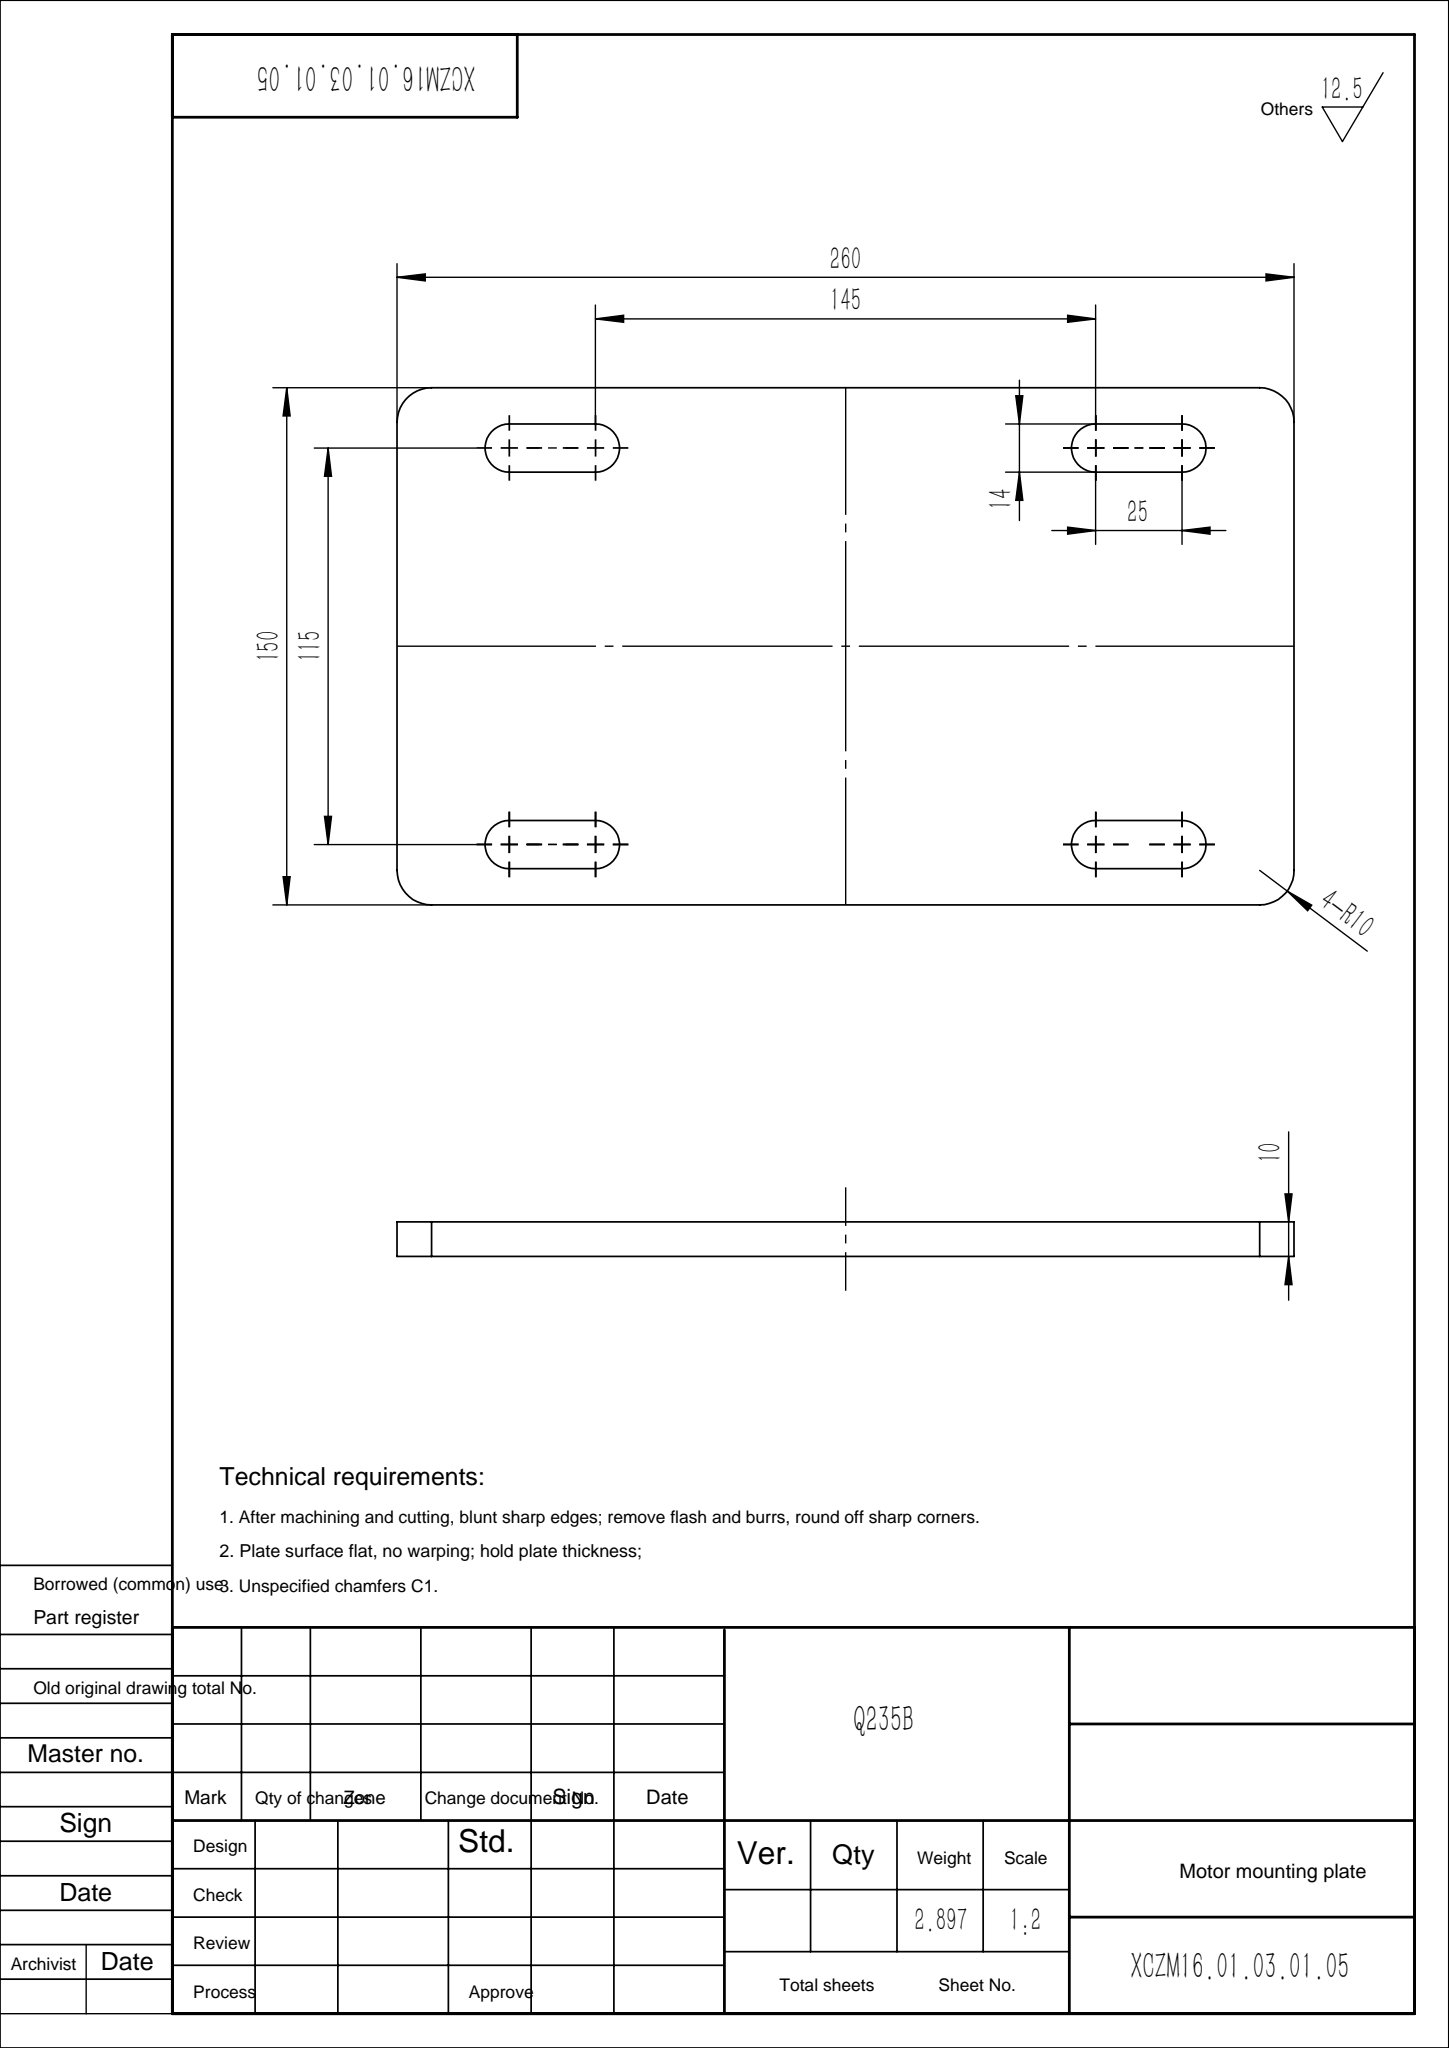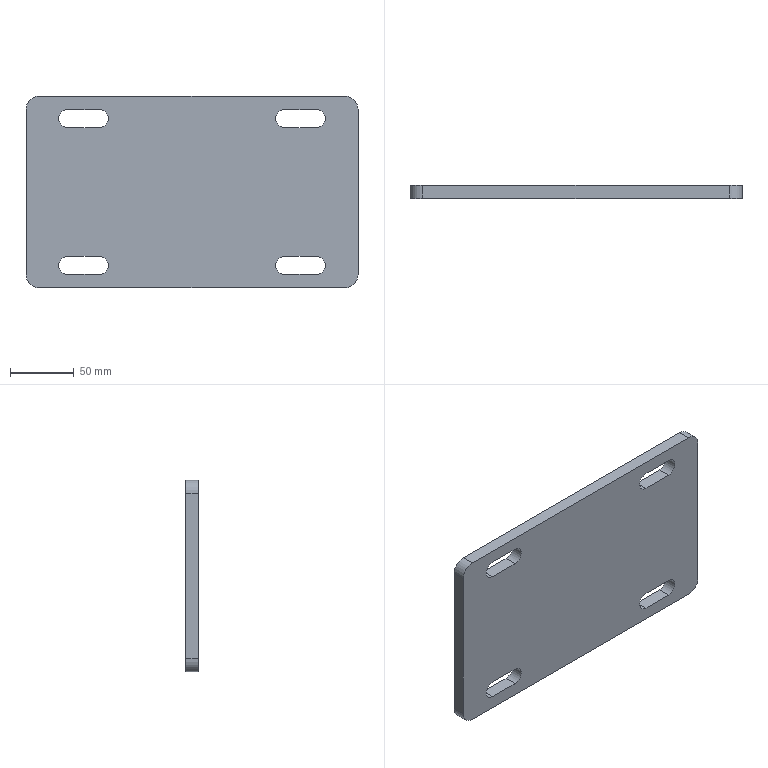Part | SolidWorks | features Extrusion 1 | 1 solid | 26 faces | box 260 x 10 x 150 mm | volume 368984 mm3 | plane 14 | cylinder 12 | commonest cylinder face diameters 14 x8 20 x4
STEP:
#1=CARTESIAN_POINT('',(-72.5,10.,64.5));
#2=VERTEX_POINT('',#1);
#3=CARTESIAN_POINT('',(-72.5,10.,50.5));
#4=VERTEX_POINT('',#3);
#5=CARTESIAN_POINT('',(-72.5,10.,57.5));
#6=DIRECTION('',(0.,1.,0.));
#7=DIRECTION('',(0.,0.,-1.));
#8=AXIS2_PLACEMENT_3D('',#5,#6,#7);
#9=CIRCLE('',#8,7.);
#10=EDGE_CURVE('',#2,#4,#9,.T.);
#11=ORIENTED_EDGE('',*,*,#10,.F.);
#12=CARTESIAN_POINT('',(-97.5,10.,64.5));
#13=VERTEX_POINT('',#12);
#14=CARTESIAN_POINT('',(-72.5,10.,64.5));
#15=DIRECTION('',(1.,0.,0.));
#16=VECTOR('',#15,1000.);
#17=LINE('',#14,#16);
#18=EDGE_CURVE('',#13,#2,#17,.T.);
#19=ORIENTED_EDGE('',*,*,#18,.F.);
#20=CARTESIAN_POINT('',(-97.5,10.,50.5));
#21=VERTEX_POINT('',#20);
#22=CARTESIAN_POINT('',(-97.5,10.,57.5));
#23=DIRECTION('',(0.,1.,0.));
#24=DIRECTION('',(0.,0.,-1.));
#25=AXIS2_PLACEMENT_3D('',#22,#23,#24);
#26=CIRCLE('',#25,7.);
#27=EDGE_CURVE('',#21,#13,#26,.T.);
#28=ORIENTED_EDGE('',*,*,#27,.F.);
#29=CARTESIAN_POINT('',(-72.5,10.,50.5));
#30=DIRECTION('',(-1.,0.,0.));
#31=VECTOR('',#30,1000.);
#32=LINE('',#29,#31);
#33=EDGE_CURVE('',#4,#21,#32,.T.);
#34=ORIENTED_EDGE('',*,*,#33,.F.);
#35=EDGE_LOOP('',(#11,#19,#28,#34));
#36=FACE_BOUND('',#35,.T.);
#37=CARTESIAN_POINT('',(-72.5,10.,-50.5));
#38=VERTEX_POINT('',#37);
#39=CARTESIAN_POINT('',(-72.5,10.,-64.5));
#40=VERTEX_POINT('',#39);
#41=CARTESIAN_POINT('',(-72.5,10.,-57.5));
#42=DIRECTION('',(0.,1.,0.));
#43=DIRECTION('',(0.,0.,1.));
#44=AXIS2_PLACEMENT_3D('',#41,#42,#43);
#45=CIRCLE('',#44,7.);
#46=EDGE_CURVE('',#38,#40,#45,.T.);
#47=ORIENTED_EDGE('',*,*,#46,.F.);
#48=CARTESIAN_POINT('',(-97.5,10.,-50.5));
#49=VERTEX_POINT('',#48);
#50=CARTESIAN_POINT('',(-72.5,10.,-50.5));
#51=DIRECTION('',(1.,0.,0.));
#52=VECTOR('',#51,1000.);
#53=LINE('',#50,#52);
#54=EDGE_CURVE('',#49,#38,#53,.T.);
#55=ORIENTED_EDGE('',*,*,#54,.F.);
#56=CARTESIAN_POINT('',(-97.5,10.,-64.5));
#57=VERTEX_POINT('',#56);
#58=CARTESIAN_POINT('',(-97.5,10.,-57.5));
#59=DIRECTION('',(0.,1.,0.));
#60=DIRECTION('',(0.,0.,1.));
#61=AXIS2_PLACEMENT_3D('',#58,#59,#60);
#62=CIRCLE('',#61,7.);
#63=EDGE_CURVE('',#57,#49,#62,.T.);
#64=ORIENTED_EDGE('',*,*,#63,.F.);
#65=CARTESIAN_POINT('',(-72.5,10.,-64.5));
#66=DIRECTION('',(-1.,0.,0.));
#67=VECTOR('',#66,1000.);
#68=LINE('',#65,#67);
#69=EDGE_CURVE('',#40,#57,#68,.T.);
#70=ORIENTED_EDGE('',*,*,#69,.F.);
#71=EDGE_LOOP('',(#47,#55,#64,#70));
#72=FACE_BOUND('',#71,.T.);
#73=CARTESIAN_POINT('',(-130.,10.,65.));
#74=VERTEX_POINT('',#73);
#75=CARTESIAN_POINT('',(-120.,10.,75.));
#76=VERTEX_POINT('',#75);
#77=CARTESIAN_POINT('',(-120.,10.,65.));
#78=DIRECTION('',(0.,1.,0.));
#79=DIRECTION('',(0.,0.,-1.));
#80=AXIS2_PLACEMENT_3D('',#77,#78,#79);
#81=CIRCLE('',#80,10.);
#82=EDGE_CURVE('',#74,#76,#81,.T.);
#83=ORIENTED_EDGE('',*,*,#82,.T.);
#84=CARTESIAN_POINT('',(120.,10.,75.));
#85=VERTEX_POINT('',#84);
#86=CARTESIAN_POINT('',(120.,10.,75.));
#87=DIRECTION('',(1.,0.,0.));
#88=VECTOR('',#87,1000.);
#89=LINE('',#86,#88);
#90=EDGE_CURVE('',#76,#85,#89,.T.);
#91=ORIENTED_EDGE('',*,*,#90,.T.);
#92=CARTESIAN_POINT('',(130.,10.,65.));
#93=VERTEX_POINT('',#92);
#94=CARTESIAN_POINT('',(120.,10.,65.));
#95=DIRECTION('',(0.,1.,0.));
#96=DIRECTION('',(0.,0.,1.));
#97=AXIS2_PLACEMENT_3D('',#94,#95,#96);
#98=CIRCLE('',#97,10.);
#99=EDGE_CURVE('',#85,#93,#98,.T.);
#100=ORIENTED_EDGE('',*,*,#99,.T.);
#101=CARTESIAN_POINT('',(130.,10.,-65.));
#102=VERTEX_POINT('',#101);
#103=CARTESIAN_POINT('',(130.,10.,65.));
#104=DIRECTION('',(0.,0.,-1.));
#105=VECTOR('',#104,1000.);
#106=LINE('',#103,#105);
#107=EDGE_CURVE('',#93,#102,#106,.T.);
#108=ORIENTED_EDGE('',*,*,#107,.T.);
#109=CARTESIAN_POINT('',(120.,10.,-75.));
#110=VERTEX_POINT('',#109);
#111=CARTESIAN_POINT('',(120.,10.,-65.));
#112=DIRECTION('',(0.,1.,0.));
#113=DIRECTION('',(0.,0.,1.));
#114=AXIS2_PLACEMENT_3D('',#111,#112,#113);
#115=CIRCLE('',#114,10.);
#116=EDGE_CURVE('',#102,#110,#115,.T.);
#117=ORIENTED_EDGE('',*,*,#116,.T.);
#118=CARTESIAN_POINT('',(-120.,10.,-75.));
#119=VERTEX_POINT('',#118);
#120=CARTESIAN_POINT('',(120.,10.,-75.));
#121=DIRECTION('',(-1.,0.,0.));
#122=VECTOR('',#121,1000.);
#123=LINE('',#120,#122);
#124=EDGE_CURVE('',#110,#119,#123,.T.);
#125=ORIENTED_EDGE('',*,*,#124,.T.);
#126=CARTESIAN_POINT('',(-130.,10.,-65.));
#127=VERTEX_POINT('',#126);
#128=CARTESIAN_POINT('',(-120.,10.,-65.));
#129=DIRECTION('',(0.,1.,0.));
#130=DIRECTION('',(0.,0.,1.));
#131=AXIS2_PLACEMENT_3D('',#128,#129,#130);
#132=CIRCLE('',#131,10.);
#133=EDGE_CURVE('',#119,#127,#132,.T.);
#134=ORIENTED_EDGE('',*,*,#133,.T.);
#135=CARTESIAN_POINT('',(-130.,10.,65.));
#136=DIRECTION('',(0.,0.,1.));
#137=VECTOR('',#136,1000.);
#138=LINE('',#135,#137);
#139=EDGE_CURVE('',#127,#74,#138,.T.);
#140=ORIENTED_EDGE('',*,*,#139,.T.);
#141=EDGE_LOOP('',(#83,#91,#100,#108,#117,#125,#134,#140));
#142=FACE_OUTER_BOUND('',#141,.T.);
#143=CARTESIAN_POINT('',(72.5,10.,-64.5));
#144=VERTEX_POINT('',#143);
#145=CARTESIAN_POINT('',(72.5,10.,-50.5));
#146=VERTEX_POINT('',#145);
#147=CARTESIAN_POINT('',(72.5,10.,-57.5));
#148=DIRECTION('',(0.,1.,0.));
#149=DIRECTION('',(0.,0.,-1.));
#150=AXIS2_PLACEMENT_3D('',#147,#148,#149);
#151=CIRCLE('',#150,7.);
#152=EDGE_CURVE('',#144,#146,#151,.T.);
#153=ORIENTED_EDGE('',*,*,#152,.F.);
#154=CARTESIAN_POINT('',(97.5,10.,-64.5));
#155=VERTEX_POINT('',#154);
#156=CARTESIAN_POINT('',(72.5,10.,-64.5));
#157=DIRECTION('',(-1.,0.,0.));
#158=VECTOR('',#157,1000.);
#159=LINE('',#156,#158);
#160=EDGE_CURVE('',#155,#144,#159,.T.);
#161=ORIENTED_EDGE('',*,*,#160,.F.);
#162=CARTESIAN_POINT('',(97.5,10.,-50.5));
#163=VERTEX_POINT('',#162);
#164=CARTESIAN_POINT('',(97.5,10.,-57.5));
#165=DIRECTION('',(0.,1.,0.));
#166=DIRECTION('',(0.,0.,-1.));
#167=AXIS2_PLACEMENT_3D('',#164,#165,#166);
#168=CIRCLE('',#167,7.);
#169=EDGE_CURVE('',#163,#155,#168,.T.);
#170=ORIENTED_EDGE('',*,*,#169,.F.);
#171=CARTESIAN_POINT('',(72.5,10.,-50.5));
#172=DIRECTION('',(1.,0.,0.));
#173=VECTOR('',#172,1000.);
#174=LINE('',#171,#173);
#175=EDGE_CURVE('',#146,#163,#174,.T.);
#176=ORIENTED_EDGE('',*,*,#175,.F.);
#177=EDGE_LOOP('',(#153,#161,#170,#176));
#178=FACE_BOUND('',#177,.T.);
#179=CARTESIAN_POINT('',(72.5,10.,50.5));
#180=VERTEX_POINT('',#179);
#181=CARTESIAN_POINT('',(72.5,10.,64.5));
#182=VERTEX_POINT('',#181);
#183=CARTESIAN_POINT('',(72.5,10.,57.5));
#184=DIRECTION('',(0.,1.,0.));
#185=DIRECTION('',(0.,0.,1.));
#186=AXIS2_PLACEMENT_3D('',#183,#184,#185);
#187=CIRCLE('',#186,7.);
#188=EDGE_CURVE('',#180,#182,#187,.T.);
#189=ORIENTED_EDGE('',*,*,#188,.F.);
#190=CARTESIAN_POINT('',(97.5,10.,50.5));
#191=VERTEX_POINT('',#190);
#192=CARTESIAN_POINT('',(72.5,10.,50.5));
#193=DIRECTION('',(-1.,0.,0.));
#194=VECTOR('',#193,1000.);
#195=LINE('',#192,#194);
#196=EDGE_CURVE('',#191,#180,#195,.T.);
#197=ORIENTED_EDGE('',*,*,#196,.F.);
#198=CARTESIAN_POINT('',(97.5,10.,64.5));
#199=VERTEX_POINT('',#198);
#200=CARTESIAN_POINT('',(97.5,10.,57.5));
#201=DIRECTION('',(0.,1.,0.));
#202=DIRECTION('',(0.,0.,1.));
#203=AXIS2_PLACEMENT_3D('',#200,#201,#202);
#204=CIRCLE('',#203,7.);
#205=EDGE_CURVE('',#199,#191,#204,.T.);
#206=ORIENTED_EDGE('',*,*,#205,.F.);
#207=CARTESIAN_POINT('',(72.5,10.,64.5));
#208=DIRECTION('',(1.,0.,0.));
#209=VECTOR('',#208,1000.);
#210=LINE('',#207,#209);
#211=EDGE_CURVE('',#182,#199,#210,.T.);
#212=ORIENTED_EDGE('',*,*,#211,.F.);
#213=EDGE_LOOP('',(#189,#197,#206,#212));
#214=FACE_BOUND('',#213,.T.);
#215=CARTESIAN_POINT('',(-120.,10.,65.));
#216=DIRECTION('',(0.,-1.,0.));
#217=DIRECTION('',(0.,0.,-1.));
#218=AXIS2_PLACEMENT_3D('',#215,#216,#217);
#219=PLANE('',#218);
#220=ADVANCED_FACE('',(#36,#72,#142,#178,#214),#219,.F.);
#221=CARTESIAN_POINT('',(-130.,0.,65.));
#222=VERTEX_POINT('',#221);
#223=CARTESIAN_POINT('',(-120.,0.,75.));
#224=VERTEX_POINT('',#223);
#225=CARTESIAN_POINT('',(-120.,0.,65.));
#226=DIRECTION('',(0.,1.,0.));
#227=DIRECTION('',(0.,0.,-1.));
#228=AXIS2_PLACEMENT_3D('',#225,#226,#227);
#229=CIRCLE('',#228,10.);
#230=EDGE_CURVE('',#222,#224,#229,.T.);
#231=ORIENTED_EDGE('',*,*,#230,.F.);
#232=CARTESIAN_POINT('',(-130.,0.,-65.));
#233=VERTEX_POINT('',#232);
#234=CARTESIAN_POINT('',(-130.,0.,65.));
#235=DIRECTION('',(0.,0.,1.));
#236=VECTOR('',#235,1000.);
#237=LINE('',#234,#236);
#238=EDGE_CURVE('',#233,#222,#237,.T.);
#239=ORIENTED_EDGE('',*,*,#238,.F.);
#240=CARTESIAN_POINT('',(-120.,0.,-75.));
#241=VERTEX_POINT('',#240);
#242=CARTESIAN_POINT('',(-120.,0.,-65.));
#243=DIRECTION('',(0.,1.,0.));
#244=DIRECTION('',(0.,0.,1.));
#245=AXIS2_PLACEMENT_3D('',#242,#243,#244);
#246=CIRCLE('',#245,10.);
#247=EDGE_CURVE('',#241,#233,#246,.T.);
#248=ORIENTED_EDGE('',*,*,#247,.F.);
#249=CARTESIAN_POINT('',(120.,0.,-75.));
#250=VERTEX_POINT('',#249);
#251=CARTESIAN_POINT('',(120.,0.,-75.));
#252=DIRECTION('',(-1.,0.,0.));
#253=VECTOR('',#252,1000.);
#254=LINE('',#251,#253);
#255=EDGE_CURVE('',#250,#241,#254,.T.);
#256=ORIENTED_EDGE('',*,*,#255,.F.);
#257=CARTESIAN_POINT('',(130.,0.,-65.));
#258=VERTEX_POINT('',#257);
#259=CARTESIAN_POINT('',(120.,0.,-65.));
#260=DIRECTION('',(0.,1.,0.));
#261=DIRECTION('',(0.,0.,1.));
#262=AXIS2_PLACEMENT_3D('',#259,#260,#261);
#263=CIRCLE('',#262,10.);
#264=EDGE_CURVE('',#258,#250,#263,.T.);
#265=ORIENTED_EDGE('',*,*,#264,.F.);
#266=CARTESIAN_POINT('',(130.,0.,65.));
#267=VERTEX_POINT('',#266);
#268=CARTESIAN_POINT('',(130.,0.,65.));
#269=DIRECTION('',(0.,0.,-1.));
#270=VECTOR('',#269,1000.);
#271=LINE('',#268,#270);
#272=EDGE_CURVE('',#267,#258,#271,.T.);
#273=ORIENTED_EDGE('',*,*,#272,.F.);
#274=CARTESIAN_POINT('',(120.,0.,75.));
#275=VERTEX_POINT('',#274);
#276=CARTESIAN_POINT('',(120.,0.,65.));
#277=DIRECTION('',(0.,1.,0.));
#278=DIRECTION('',(0.,0.,1.));
#279=AXIS2_PLACEMENT_3D('',#276,#277,#278);
#280=CIRCLE('',#279,10.);
#281=EDGE_CURVE('',#275,#267,#280,.T.);
#282=ORIENTED_EDGE('',*,*,#281,.F.);
#283=CARTESIAN_POINT('',(120.,0.,75.));
#284=DIRECTION('',(1.,0.,0.));
#285=VECTOR('',#284,1000.);
#286=LINE('',#283,#285);
#287=EDGE_CURVE('',#224,#275,#286,.T.);
#288=ORIENTED_EDGE('',*,*,#287,.F.);
#289=EDGE_LOOP('',(#231,#239,#248,#256,#265,#273,#282,#288));
#290=FACE_OUTER_BOUND('',#289,.T.);
#291=CARTESIAN_POINT('',(-97.5,0.,-50.5));
#292=VERTEX_POINT('',#291);
#293=CARTESIAN_POINT('',(-72.5,0.,-50.5));
#294=VERTEX_POINT('',#293);
#295=CARTESIAN_POINT('',(-72.5,0.,-50.5));
#296=DIRECTION('',(1.,0.,0.));
#297=VECTOR('',#296,1000.);
#298=LINE('',#295,#297);
#299=EDGE_CURVE('',#292,#294,#298,.T.);
#300=ORIENTED_EDGE('',*,*,#299,.T.);
#301=CARTESIAN_POINT('',(-72.5,0.,-64.5));
#302=VERTEX_POINT('',#301);
#303=CARTESIAN_POINT('',(-72.5,0.,-57.5));
#304=DIRECTION('',(0.,1.,0.));
#305=DIRECTION('',(0.,0.,1.));
#306=AXIS2_PLACEMENT_3D('',#303,#304,#305);
#307=CIRCLE('',#306,7.);
#308=EDGE_CURVE('',#294,#302,#307,.T.);
#309=ORIENTED_EDGE('',*,*,#308,.T.);
#310=CARTESIAN_POINT('',(-97.5,0.,-64.5));
#311=VERTEX_POINT('',#310);
#312=CARTESIAN_POINT('',(-72.5,0.,-64.5));
#313=DIRECTION('',(-1.,0.,0.));
#314=VECTOR('',#313,1000.);
#315=LINE('',#312,#314);
#316=EDGE_CURVE('',#302,#311,#315,.T.);
#317=ORIENTED_EDGE('',*,*,#316,.T.);
#318=CARTESIAN_POINT('',(-97.5,0.,-57.5));
#319=DIRECTION('',(0.,1.,0.));
#320=DIRECTION('',(0.,0.,1.));
#321=AXIS2_PLACEMENT_3D('',#318,#319,#320);
#322=CIRCLE('',#321,7.);
#323=EDGE_CURVE('',#311,#292,#322,.T.);
#324=ORIENTED_EDGE('',*,*,#323,.T.);
#325=EDGE_LOOP('',(#300,#309,#317,#324));
#326=FACE_BOUND('',#325,.T.);
#327=CARTESIAN_POINT('',(97.5,0.,-64.5));
#328=VERTEX_POINT('',#327);
#329=CARTESIAN_POINT('',(72.5,0.,-64.5));
#330=VERTEX_POINT('',#329);
#331=CARTESIAN_POINT('',(72.5,0.,-64.5));
#332=DIRECTION('',(-1.,0.,0.));
#333=VECTOR('',#332,1000.);
#334=LINE('',#331,#333);
#335=EDGE_CURVE('',#328,#330,#334,.T.);
#336=ORIENTED_EDGE('',*,*,#335,.T.);
#337=CARTESIAN_POINT('',(72.5,0.,-50.5));
#338=VERTEX_POINT('',#337);
#339=CARTESIAN_POINT('',(72.5,0.,-57.5));
#340=DIRECTION('',(0.,1.,0.));
#341=DIRECTION('',(0.,0.,-1.));
#342=AXIS2_PLACEMENT_3D('',#339,#340,#341);
#343=CIRCLE('',#342,7.);
#344=EDGE_CURVE('',#330,#338,#343,.T.);
#345=ORIENTED_EDGE('',*,*,#344,.T.);
#346=CARTESIAN_POINT('',(97.5,0.,-50.5));
#347=VERTEX_POINT('',#346);
#348=CARTESIAN_POINT('',(72.5,0.,-50.5));
#349=DIRECTION('',(1.,0.,0.));
#350=VECTOR('',#349,1000.);
#351=LINE('',#348,#350);
#352=EDGE_CURVE('',#338,#347,#351,.T.);
#353=ORIENTED_EDGE('',*,*,#352,.T.);
#354=CARTESIAN_POINT('',(97.5,0.,-57.5));
#355=DIRECTION('',(0.,1.,0.));
#356=DIRECTION('',(0.,0.,-1.));
#357=AXIS2_PLACEMENT_3D('',#354,#355,#356);
#358=CIRCLE('',#357,7.);
#359=EDGE_CURVE('',#347,#328,#358,.T.);
#360=ORIENTED_EDGE('',*,*,#359,.T.);
#361=EDGE_LOOP('',(#336,#345,#353,#360));
#362=FACE_BOUND('',#361,.T.);
#363=CARTESIAN_POINT('',(-97.5,0.,64.5));
#364=VERTEX_POINT('',#363);
#365=CARTESIAN_POINT('',(-72.5,0.,64.5));
#366=VERTEX_POINT('',#365);
#367=CARTESIAN_POINT('',(-72.5,0.,64.5));
#368=DIRECTION('',(1.,0.,0.));
#369=VECTOR('',#368,1000.);
#370=LINE('',#367,#369);
#371=EDGE_CURVE('',#364,#366,#370,.T.);
#372=ORIENTED_EDGE('',*,*,#371,.T.);
#373=CARTESIAN_POINT('',(-72.5,0.,50.5));
#374=VERTEX_POINT('',#373);
#375=CARTESIAN_POINT('',(-72.5,0.,57.5));
#376=DIRECTION('',(0.,1.,0.));
#377=DIRECTION('',(0.,0.,-1.));
#378=AXIS2_PLACEMENT_3D('',#375,#376,#377);
#379=CIRCLE('',#378,7.);
#380=EDGE_CURVE('',#366,#374,#379,.T.);
#381=ORIENTED_EDGE('',*,*,#380,.T.);
#382=CARTESIAN_POINT('',(-97.5,0.,50.5));
#383=VERTEX_POINT('',#382);
#384=CARTESIAN_POINT('',(-72.5,0.,50.5));
#385=DIRECTION('',(-1.,0.,0.));
#386=VECTOR('',#385,1000.);
#387=LINE('',#384,#386);
#388=EDGE_CURVE('',#374,#383,#387,.T.);
#389=ORIENTED_EDGE('',*,*,#388,.T.);
#390=CARTESIAN_POINT('',(-97.5,0.,57.5));
#391=DIRECTION('',(0.,1.,0.));
#392=DIRECTION('',(0.,0.,-1.));
#393=AXIS2_PLACEMENT_3D('',#390,#391,#392);
#394=CIRCLE('',#393,7.);
#395=EDGE_CURVE('',#383,#364,#394,.T.);
#396=ORIENTED_EDGE('',*,*,#395,.T.);
#397=EDGE_LOOP('',(#372,#381,#389,#396));
#398=FACE_BOUND('',#397,.T.);
#399=CARTESIAN_POINT('',(97.5,0.,50.5));
#400=VERTEX_POINT('',#399);
#401=CARTESIAN_POINT('',(72.5,0.,50.5));
#402=VERTEX_POINT('',#401);
#403=CARTESIAN_POINT('',(72.5,0.,50.5));
#404=DIRECTION('',(-1.,0.,0.));
#405=VECTOR('',#404,1000.);
#406=LINE('',#403,#405);
#407=EDGE_CURVE('',#400,#402,#406,.T.);
#408=ORIENTED_EDGE('',*,*,#407,.T.);
#409=CARTESIAN_POINT('',(72.5,0.,64.5));
#410=VERTEX_POINT('',#409);
#411=CARTESIAN_POINT('',(72.5,0.,57.5));
#412=DIRECTION('',(0.,1.,0.));
#413=DIRECTION('',(0.,0.,1.));
#414=AXIS2_PLACEMENT_3D('',#411,#412,#413);
#415=CIRCLE('',#414,7.);
#416=EDGE_CURVE('',#402,#410,#415,.T.);
#417=ORIENTED_EDGE('',*,*,#416,.T.);
#418=CARTESIAN_POINT('',(97.5,0.,64.5));
#419=VERTEX_POINT('',#418);
#420=CARTESIAN_POINT('',(72.5,0.,64.5));
#421=DIRECTION('',(1.,0.,0.));
#422=VECTOR('',#421,1000.);
#423=LINE('',#420,#422);
#424=EDGE_CURVE('',#410,#419,#423,.T.);
#425=ORIENTED_EDGE('',*,*,#424,.T.);
#426=CARTESIAN_POINT('',(97.5,0.,57.5));
#427=DIRECTION('',(0.,1.,0.));
#428=DIRECTION('',(0.,0.,1.));
#429=AXIS2_PLACEMENT_3D('',#426,#427,#428);
#430=CIRCLE('',#429,7.);
#431=EDGE_CURVE('',#419,#400,#430,.T.);
#432=ORIENTED_EDGE('',*,*,#431,.T.);
#433=EDGE_LOOP('',(#408,#417,#425,#432));
#434=FACE_BOUND('',#433,.T.);
#435=CARTESIAN_POINT('',(-120.,0.,65.));
#436=DIRECTION('',(0.,-1.,0.));
#437=DIRECTION('',(0.,0.,-1.));
#438=AXIS2_PLACEMENT_3D('',#435,#436,#437);
#439=PLANE('',#438);
#440=ADVANCED_FACE('',(#290,#326,#362,#398,#434),#439,.T.);
#441=ORIENTED_EDGE('',*,*,#230,.T.);
#442=CARTESIAN_POINT('',(-120.,10.,75.));
#443=DIRECTION('',(0.,-1.,0.));
#444=VECTOR('',#443,1000.);
#445=LINE('',#442,#444);
#446=EDGE_CURVE('',#76,#224,#445,.T.);
#447=ORIENTED_EDGE('',*,*,#446,.F.);
#448=ORIENTED_EDGE('',*,*,#82,.F.);
#449=CARTESIAN_POINT('',(-130.,10.,65.));
#450=DIRECTION('',(0.,-1.,0.));
#451=VECTOR('',#450,1000.);
#452=LINE('',#449,#451);
#453=EDGE_CURVE('',#74,#222,#452,.T.);
#454=ORIENTED_EDGE('',*,*,#453,.T.);
#455=EDGE_LOOP('',(#441,#447,#448,#454));
#456=FACE_OUTER_BOUND('',#455,.T.);
#457=CARTESIAN_POINT('',(-120.,10.,65.));
#458=DIRECTION('',(0.,-1.,0.));
#459=DIRECTION('',(0.,0.,-1.));
#460=AXIS2_PLACEMENT_3D('',#457,#458,#459);
#461=CYLINDRICAL_SURFACE('',#460,10.);
#462=ADVANCED_FACE('',(#456),#461,.T.);
#463=ORIENTED_EDGE('',*,*,#287,.T.);
#464=CARTESIAN_POINT('',(120.,10.,75.));
#465=DIRECTION('',(0.,-1.,0.));
#466=VECTOR('',#465,1000.);
#467=LINE('',#464,#466);
#468=EDGE_CURVE('',#85,#275,#467,.T.);
#469=ORIENTED_EDGE('',*,*,#468,.F.);
#470=ORIENTED_EDGE('',*,*,#90,.F.);
#471=ORIENTED_EDGE('',*,*,#446,.T.);
#472=EDGE_LOOP('',(#463,#469,#470,#471));
#473=FACE_OUTER_BOUND('',#472,.T.);
#474=CARTESIAN_POINT('',(120.,10.,75.));
#475=DIRECTION('',(0.,0.,-1.));
#476=DIRECTION('',(-1.,0.,0.));
#477=AXIS2_PLACEMENT_3D('',#474,#475,#476);
#478=PLANE('',#477);
#479=ADVANCED_FACE('',(#473),#478,.F.);
#480=ORIENTED_EDGE('',*,*,#281,.T.);
#481=CARTESIAN_POINT('',(130.,10.,65.));
#482=DIRECTION('',(0.,-1.,0.));
#483=VECTOR('',#482,1000.);
#484=LINE('',#481,#483);
#485=EDGE_CURVE('',#93,#267,#484,.T.);
#486=ORIENTED_EDGE('',*,*,#485,.F.);
#487=ORIENTED_EDGE('',*,*,#99,.F.);
#488=ORIENTED_EDGE('',*,*,#468,.T.);
#489=EDGE_LOOP('',(#480,#486,#487,#488));
#490=FACE_OUTER_BOUND('',#489,.T.);
#491=CARTESIAN_POINT('',(120.,10.,65.));
#492=DIRECTION('',(0.,-1.,0.));
#493=DIRECTION('',(0.,0.,-1.));
#494=AXIS2_PLACEMENT_3D('',#491,#492,#493);
#495=CYLINDRICAL_SURFACE('',#494,10.);
#496=ADVANCED_FACE('',(#490),#495,.T.);
#497=ORIENTED_EDGE('',*,*,#272,.T.);
#498=CARTESIAN_POINT('',(130.,10.,-65.));
#499=DIRECTION('',(0.,-1.,0.));
#500=VECTOR('',#499,1000.);
#501=LINE('',#498,#500);
#502=EDGE_CURVE('',#102,#258,#501,.T.);
#503=ORIENTED_EDGE('',*,*,#502,.F.);
#504=ORIENTED_EDGE('',*,*,#107,.F.);
#505=ORIENTED_EDGE('',*,*,#485,.T.);
#506=EDGE_LOOP('',(#497,#503,#504,#505));
#507=FACE_OUTER_BOUND('',#506,.T.);
#508=CARTESIAN_POINT('',(130.,10.,65.));
#509=DIRECTION('',(-1.,0.,0.));
#510=DIRECTION('',(0.,0.,1.));
#511=AXIS2_PLACEMENT_3D('',#508,#509,#510);
#512=PLANE('',#511);
#513=ADVANCED_FACE('',(#507),#512,.F.);
#514=ORIENTED_EDGE('',*,*,#264,.T.);
#515=CARTESIAN_POINT('',(120.,10.,-75.));
#516=DIRECTION('',(0.,-1.,0.));
#517=VECTOR('',#516,1000.);
#518=LINE('',#515,#517);
#519=EDGE_CURVE('',#110,#250,#518,.T.);
#520=ORIENTED_EDGE('',*,*,#519,.F.);
#521=ORIENTED_EDGE('',*,*,#116,.F.);
#522=ORIENTED_EDGE('',*,*,#502,.T.);
#523=EDGE_LOOP('',(#514,#520,#521,#522));
#524=FACE_OUTER_BOUND('',#523,.T.);
#525=CARTESIAN_POINT('',(120.,10.,-65.));
#526=DIRECTION('',(0.,-1.,0.));
#527=DIRECTION('',(0.,0.,-1.));
#528=AXIS2_PLACEMENT_3D('',#525,#526,#527);
#529=CYLINDRICAL_SURFACE('',#528,10.);
#530=ADVANCED_FACE('',(#524),#529,.T.);
#531=ORIENTED_EDGE('',*,*,#255,.T.);
#532=CARTESIAN_POINT('',(-120.,10.,-75.));
#533=DIRECTION('',(0.,-1.,0.));
#534=VECTOR('',#533,1000.);
#535=LINE('',#532,#534);
#536=EDGE_CURVE('',#119,#241,#535,.T.);
#537=ORIENTED_EDGE('',*,*,#536,.F.);
#538=ORIENTED_EDGE('',*,*,#124,.F.);
#539=ORIENTED_EDGE('',*,*,#519,.T.);
#540=EDGE_LOOP('',(#531,#537,#538,#539));
#541=FACE_OUTER_BOUND('',#540,.T.);
#542=CARTESIAN_POINT('',(120.,10.,-75.));
#543=DIRECTION('',(0.,0.,1.));
#544=DIRECTION('',(1.,0.,0.));
#545=AXIS2_PLACEMENT_3D('',#542,#543,#544);
#546=PLANE('',#545);
#547=ADVANCED_FACE('',(#541),#546,.F.);
#548=ORIENTED_EDGE('',*,*,#247,.T.);
#549=CARTESIAN_POINT('',(-130.,10.,-65.));
#550=DIRECTION('',(0.,-1.,0.));
#551=VECTOR('',#550,1000.);
#552=LINE('',#549,#551);
#553=EDGE_CURVE('',#127,#233,#552,.T.);
#554=ORIENTED_EDGE('',*,*,#553,.F.);
#555=ORIENTED_EDGE('',*,*,#133,.F.);
#556=ORIENTED_EDGE('',*,*,#536,.T.);
#557=EDGE_LOOP('',(#548,#554,#555,#556));
#558=FACE_OUTER_BOUND('',#557,.T.);
#559=CARTESIAN_POINT('',(-120.,10.,-65.));
#560=DIRECTION('',(0.,-1.,0.));
#561=DIRECTION('',(0.,0.,-1.));
#562=AXIS2_PLACEMENT_3D('',#559,#560,#561);
#563=CYLINDRICAL_SURFACE('',#562,10.);
#564=ADVANCED_FACE('',(#558),#563,.T.);
#565=ORIENTED_EDGE('',*,*,#238,.T.);
#566=ORIENTED_EDGE('',*,*,#453,.F.);
#567=ORIENTED_EDGE('',*,*,#139,.F.);
#568=ORIENTED_EDGE('',*,*,#553,.T.);
#569=EDGE_LOOP('',(#565,#566,#567,#568));
#570=FACE_OUTER_BOUND('',#569,.T.);
#571=CARTESIAN_POINT('',(-130.,10.,65.));
#572=DIRECTION('',(1.,0.,0.));
#573=DIRECTION('',(0.,0.,-1.));
#574=AXIS2_PLACEMENT_3D('',#571,#572,#573);
#575=PLANE('',#574);
#576=ADVANCED_FACE('',(#570),#575,.F.);
#577=ORIENTED_EDGE('',*,*,#308,.F.);
#578=CARTESIAN_POINT('',(-72.5,10.,-50.5));
#579=DIRECTION('',(0.,-1.,0.));
#580=VECTOR('',#579,1000.);
#581=LINE('',#578,#580);
#582=EDGE_CURVE('',#38,#294,#581,.T.);
#583=ORIENTED_EDGE('',*,*,#582,.F.);
#584=ORIENTED_EDGE('',*,*,#46,.T.);
#585=CARTESIAN_POINT('',(-72.5,10.,-64.5));
#586=DIRECTION('',(0.,-1.,0.));
#587=VECTOR('',#586,1000.);
#588=LINE('',#585,#587);
#589=EDGE_CURVE('',#40,#302,#588,.T.);
#590=ORIENTED_EDGE('',*,*,#589,.T.);
#591=EDGE_LOOP('',(#577,#583,#584,#590));
#592=FACE_OUTER_BOUND('',#591,.T.);
#593=CARTESIAN_POINT('',(-72.5,10.,-57.5));
#594=DIRECTION('',(0.,-1.,0.));
#595=DIRECTION('',(0.,0.,-1.));
#596=AXIS2_PLACEMENT_3D('',#593,#594,#595);
#597=CYLINDRICAL_SURFACE('',#596,7.);
#598=ADVANCED_FACE('',(#592),#597,.F.);
#599=ORIENTED_EDGE('',*,*,#316,.F.);
#600=ORIENTED_EDGE('',*,*,#589,.F.);
#601=ORIENTED_EDGE('',*,*,#69,.T.);
#602=CARTESIAN_POINT('',(-97.5,10.,-64.5));
#603=DIRECTION('',(0.,-1.,0.));
#604=VECTOR('',#603,1000.);
#605=LINE('',#602,#604);
#606=EDGE_CURVE('',#57,#311,#605,.T.);
#607=ORIENTED_EDGE('',*,*,#606,.T.);
#608=EDGE_LOOP('',(#599,#600,#601,#607));
#609=FACE_OUTER_BOUND('',#608,.T.);
#610=CARTESIAN_POINT('',(-72.5,10.,-64.5));
#611=DIRECTION('',(0.,0.,1.));
#612=DIRECTION('',(1.,0.,0.));
#613=AXIS2_PLACEMENT_3D('',#610,#611,#612);
#614=PLANE('',#613);
#615=ADVANCED_FACE('',(#609),#614,.T.);
#616=ORIENTED_EDGE('',*,*,#323,.F.);
#617=ORIENTED_EDGE('',*,*,#606,.F.);
#618=ORIENTED_EDGE('',*,*,#63,.T.);
#619=CARTESIAN_POINT('',(-97.5,10.,-50.5));
#620=DIRECTION('',(0.,-1.,0.));
#621=VECTOR('',#620,1000.);
#622=LINE('',#619,#621);
#623=EDGE_CURVE('',#49,#292,#622,.T.);
#624=ORIENTED_EDGE('',*,*,#623,.T.);
#625=EDGE_LOOP('',(#616,#617,#618,#624));
#626=FACE_OUTER_BOUND('',#625,.T.);
#627=CARTESIAN_POINT('',(-97.5,10.,-57.5));
#628=DIRECTION('',(0.,-1.,0.));
#629=DIRECTION('',(0.,0.,-1.));
#630=AXIS2_PLACEMENT_3D('',#627,#628,#629);
#631=CYLINDRICAL_SURFACE('',#630,7.);
#632=ADVANCED_FACE('',(#626),#631,.F.);
#633=ORIENTED_EDGE('',*,*,#299,.F.);
#634=ORIENTED_EDGE('',*,*,#623,.F.);
#635=ORIENTED_EDGE('',*,*,#54,.T.);
#636=ORIENTED_EDGE('',*,*,#582,.T.);
#637=EDGE_LOOP('',(#633,#634,#635,#636));
#638=FACE_OUTER_BOUND('',#637,.T.);
#639=CARTESIAN_POINT('',(-72.5,10.,-50.5));
#640=DIRECTION('',(0.,0.,-1.));
#641=DIRECTION('',(-1.,0.,0.));
#642=AXIS2_PLACEMENT_3D('',#639,#640,#641);
#643=PLANE('',#642);
#644=ADVANCED_FACE('',(#638),#643,.T.);
#645=ORIENTED_EDGE('',*,*,#344,.F.);
#646=CARTESIAN_POINT('',(72.5,10.,-64.5));
#647=DIRECTION('',(0.,-1.,0.));
#648=VECTOR('',#647,1000.);
#649=LINE('',#646,#648);
#650=EDGE_CURVE('',#144,#330,#649,.T.);
#651=ORIENTED_EDGE('',*,*,#650,.F.);
#652=ORIENTED_EDGE('',*,*,#152,.T.);
#653=CARTESIAN_POINT('',(72.5,10.,-50.5));
#654=DIRECTION('',(0.,-1.,0.));
#655=VECTOR('',#654,1000.);
#656=LINE('',#653,#655);
#657=EDGE_CURVE('',#146,#338,#656,.T.);
#658=ORIENTED_EDGE('',*,*,#657,.T.);
#659=EDGE_LOOP('',(#645,#651,#652,#658));
#660=FACE_OUTER_BOUND('',#659,.T.);
#661=CARTESIAN_POINT('',(72.5,10.,-57.5));
#662=DIRECTION('',(0.,-1.,0.));
#663=DIRECTION('',(0.,0.,-1.));
#664=AXIS2_PLACEMENT_3D('',#661,#662,#663);
#665=CYLINDRICAL_SURFACE('',#664,7.);
#666=ADVANCED_FACE('',(#660),#665,.F.);
#667=ORIENTED_EDGE('',*,*,#352,.F.);
#668=ORIENTED_EDGE('',*,*,#657,.F.);
#669=ORIENTED_EDGE('',*,*,#175,.T.);
#670=CARTESIAN_POINT('',(97.5,10.,-50.5));
#671=DIRECTION('',(0.,-1.,0.));
#672=VECTOR('',#671,1000.);
#673=LINE('',#670,#672);
#674=EDGE_CURVE('',#163,#347,#673,.T.);
#675=ORIENTED_EDGE('',*,*,#674,.T.);
#676=EDGE_LOOP('',(#667,#668,#669,#675));
#677=FACE_OUTER_BOUND('',#676,.T.);
#678=CARTESIAN_POINT('',(72.5,10.,-50.5));
#679=DIRECTION('',(0.,0.,-1.));
#680=DIRECTION('',(-1.,0.,0.));
#681=AXIS2_PLACEMENT_3D('',#678,#679,#680);
#682=PLANE('',#681);
#683=ADVANCED_FACE('',(#677),#682,.T.);
#684=ORIENTED_EDGE('',*,*,#359,.F.);
#685=ORIENTED_EDGE('',*,*,#674,.F.);
#686=ORIENTED_EDGE('',*,*,#169,.T.);
#687=CARTESIAN_POINT('',(97.5,10.,-64.5));
#688=DIRECTION('',(0.,-1.,0.));
#689=VECTOR('',#688,1000.);
#690=LINE('',#687,#689);
#691=EDGE_CURVE('',#155,#328,#690,.T.);
#692=ORIENTED_EDGE('',*,*,#691,.T.);
#693=EDGE_LOOP('',(#684,#685,#686,#692));
#694=FACE_OUTER_BOUND('',#693,.T.);
#695=CARTESIAN_POINT('',(97.5,10.,-57.5));
#696=DIRECTION('',(0.,-1.,0.));
#697=DIRECTION('',(0.,0.,-1.));
#698=AXIS2_PLACEMENT_3D('',#695,#696,#697);
#699=CYLINDRICAL_SURFACE('',#698,7.);
#700=ADVANCED_FACE('',(#694),#699,.F.);
#701=ORIENTED_EDGE('',*,*,#335,.F.);
#702=ORIENTED_EDGE('',*,*,#691,.F.);
#703=ORIENTED_EDGE('',*,*,#160,.T.);
#704=ORIENTED_EDGE('',*,*,#650,.T.);
#705=EDGE_LOOP('',(#701,#702,#703,#704));
#706=FACE_OUTER_BOUND('',#705,.T.);
#707=CARTESIAN_POINT('',(72.5,10.,-64.5));
#708=DIRECTION('',(0.,0.,1.));
#709=DIRECTION('',(1.,0.,0.));
#710=AXIS2_PLACEMENT_3D('',#707,#708,#709);
#711=PLANE('',#710);
#712=ADVANCED_FACE('',(#706),#711,.T.);
#713=ORIENTED_EDGE('',*,*,#380,.F.);
#714=CARTESIAN_POINT('',(-72.5,10.,64.5));
#715=DIRECTION('',(0.,-1.,0.));
#716=VECTOR('',#715,1000.);
#717=LINE('',#714,#716);
#718=EDGE_CURVE('',#2,#366,#717,.T.);
#719=ORIENTED_EDGE('',*,*,#718,.F.);
#720=ORIENTED_EDGE('',*,*,#10,.T.);
#721=CARTESIAN_POINT('',(-72.5,10.,50.5));
#722=DIRECTION('',(0.,-1.,0.));
#723=VECTOR('',#722,1000.);
#724=LINE('',#721,#723);
#725=EDGE_CURVE('',#4,#374,#724,.T.);
#726=ORIENTED_EDGE('',*,*,#725,.T.);
#727=EDGE_LOOP('',(#713,#719,#720,#726));
#728=FACE_OUTER_BOUND('',#727,.T.);
#729=CARTESIAN_POINT('',(-72.5,10.,57.5));
#730=DIRECTION('',(0.,-1.,0.));
#731=DIRECTION('',(0.,0.,-1.));
#732=AXIS2_PLACEMENT_3D('',#729,#730,#731);
#733=CYLINDRICAL_SURFACE('',#732,7.);
#734=ADVANCED_FACE('',(#728),#733,.F.);
#735=ORIENTED_EDGE('',*,*,#388,.F.);
#736=ORIENTED_EDGE('',*,*,#725,.F.);
#737=ORIENTED_EDGE('',*,*,#33,.T.);
#738=CARTESIAN_POINT('',(-97.5,10.,50.5));
#739=DIRECTION('',(0.,-1.,0.));
#740=VECTOR('',#739,1000.);
#741=LINE('',#738,#740);
#742=EDGE_CURVE('',#21,#383,#741,.T.);
#743=ORIENTED_EDGE('',*,*,#742,.T.);
#744=EDGE_LOOP('',(#735,#736,#737,#743));
#745=FACE_OUTER_BOUND('',#744,.T.);
#746=CARTESIAN_POINT('',(-72.5,10.,50.5));
#747=DIRECTION('',(0.,0.,1.));
#748=DIRECTION('',(1.,0.,0.));
#749=AXIS2_PLACEMENT_3D('',#746,#747,#748);
#750=PLANE('',#749);
#751=ADVANCED_FACE('',(#745),#750,.T.);
#752=ORIENTED_EDGE('',*,*,#395,.F.);
#753=ORIENTED_EDGE('',*,*,#742,.F.);
#754=ORIENTED_EDGE('',*,*,#27,.T.);
#755=CARTESIAN_POINT('',(-97.5,10.,64.5));
#756=DIRECTION('',(0.,-1.,0.));
#757=VECTOR('',#756,1000.);
#758=LINE('',#755,#757);
#759=EDGE_CURVE('',#13,#364,#758,.T.);
#760=ORIENTED_EDGE('',*,*,#759,.T.);
#761=EDGE_LOOP('',(#752,#753,#754,#760));
#762=FACE_OUTER_BOUND('',#761,.T.);
#763=CARTESIAN_POINT('',(-97.5,10.,57.5));
#764=DIRECTION('',(0.,-1.,0.));
#765=DIRECTION('',(0.,0.,-1.));
#766=AXIS2_PLACEMENT_3D('',#763,#764,#765);
#767=CYLINDRICAL_SURFACE('',#766,7.);
#768=ADVANCED_FACE('',(#762),#767,.F.);
#769=ORIENTED_EDGE('',*,*,#371,.F.);
#770=ORIENTED_EDGE('',*,*,#759,.F.);
#771=ORIENTED_EDGE('',*,*,#18,.T.);
#772=ORIENTED_EDGE('',*,*,#718,.T.);
#773=EDGE_LOOP('',(#769,#770,#771,#772));
#774=FACE_OUTER_BOUND('',#773,.T.);
#775=CARTESIAN_POINT('',(-72.5,10.,64.5));
#776=DIRECTION('',(0.,0.,-1.));
#777=DIRECTION('',(-1.,0.,0.));
#778=AXIS2_PLACEMENT_3D('',#775,#776,#777);
#779=PLANE('',#778);
#780=ADVANCED_FACE('',(#774),#779,.T.);
#781=ORIENTED_EDGE('',*,*,#416,.F.);
#782=CARTESIAN_POINT('',(72.5,10.,50.5));
#783=DIRECTION('',(0.,-1.,0.));
#784=VECTOR('',#783,1000.);
#785=LINE('',#782,#784);
#786=EDGE_CURVE('',#180,#402,#785,.T.);
#787=ORIENTED_EDGE('',*,*,#786,.F.);
#788=ORIENTED_EDGE('',*,*,#188,.T.);
#789=CARTESIAN_POINT('',(72.5,10.,64.5));
#790=DIRECTION('',(0.,-1.,0.));
#791=VECTOR('',#790,1000.);
#792=LINE('',#789,#791);
#793=EDGE_CURVE('',#182,#410,#792,.T.);
#794=ORIENTED_EDGE('',*,*,#793,.T.);
#795=EDGE_LOOP('',(#781,#787,#788,#794));
#796=FACE_OUTER_BOUND('',#795,.T.);
#797=CARTESIAN_POINT('',(72.5,10.,57.5));
#798=DIRECTION('',(0.,-1.,0.));
#799=DIRECTION('',(0.,0.,-1.));
#800=AXIS2_PLACEMENT_3D('',#797,#798,#799);
#801=CYLINDRICAL_SURFACE('',#800,7.);
#802=ADVANCED_FACE('',(#796),#801,.F.);
#803=ORIENTED_EDGE('',*,*,#424,.F.);
#804=ORIENTED_EDGE('',*,*,#793,.F.);
#805=ORIENTED_EDGE('',*,*,#211,.T.);
#806=CARTESIAN_POINT('',(97.5,10.,64.5));
#807=DIRECTION('',(0.,-1.,0.));
#808=VECTOR('',#807,1000.);
#809=LINE('',#806,#808);
#810=EDGE_CURVE('',#199,#419,#809,.T.);
#811=ORIENTED_EDGE('',*,*,#810,.T.);
#812=EDGE_LOOP('',(#803,#804,#805,#811));
#813=FACE_OUTER_BOUND('',#812,.T.);
#814=CARTESIAN_POINT('',(72.5,10.,64.5));
#815=DIRECTION('',(0.,0.,-1.));
#816=DIRECTION('',(-1.,0.,0.));
#817=AXIS2_PLACEMENT_3D('',#814,#815,#816);
#818=PLANE('',#817);
#819=ADVANCED_FACE('',(#813),#818,.T.);
#820=ORIENTED_EDGE('',*,*,#431,.F.);
#821=ORIENTED_EDGE('',*,*,#810,.F.);
#822=ORIENTED_EDGE('',*,*,#205,.T.);
#823=CARTESIAN_POINT('',(97.5,10.,50.5));
#824=DIRECTION('',(0.,-1.,0.));
#825=VECTOR('',#824,1000.);
#826=LINE('',#823,#825);
#827=EDGE_CURVE('',#191,#400,#826,.T.);
#828=ORIENTED_EDGE('',*,*,#827,.T.);
#829=EDGE_LOOP('',(#820,#821,#822,#828));
#830=FACE_OUTER_BOUND('',#829,.T.);
#831=CARTESIAN_POINT('',(97.5,10.,57.5));
#832=DIRECTION('',(0.,-1.,0.));
#833=DIRECTION('',(0.,0.,-1.));
#834=AXIS2_PLACEMENT_3D('',#831,#832,#833);
#835=CYLINDRICAL_SURFACE('',#834,7.);
#836=ADVANCED_FACE('',(#830),#835,.F.);
#837=ORIENTED_EDGE('',*,*,#407,.F.);
#838=ORIENTED_EDGE('',*,*,#827,.F.);
#839=ORIENTED_EDGE('',*,*,#196,.T.);
#840=ORIENTED_EDGE('',*,*,#786,.T.);
#841=EDGE_LOOP('',(#837,#838,#839,#840));
#842=FACE_OUTER_BOUND('',#841,.T.);
#843=CARTESIAN_POINT('',(72.5,10.,50.5));
#844=DIRECTION('',(0.,0.,1.));
#845=DIRECTION('',(1.,0.,0.));
#846=AXIS2_PLACEMENT_3D('',#843,#844,#845);
#847=PLANE('',#846);
#848=ADVANCED_FACE('',(#842),#847,.T.);
#849=CLOSED_SHELL('',(#220,#440,#462,#479,#496,#513,#530,#547,#564,#576,#598,#615,#632,#644,#666,#683,#700,#712,#734,#751,#768,#780,#802,#819,#836,#848));
#850=MANIFOLD_SOLID_BREP('',#849);
#851=CARTESIAN_POINT('',(0.,0.,0.));
#852=DIRECTION('',(0.,0.,1.));
#853=DIRECTION('',(1.,0.,0.));
#854=AXIS2_PLACEMENT_3D('',#851,#852,#853);
#855=(LENGTH_UNIT()NAMED_UNIT(*)SI_UNIT(.MILLI.,.METRE.));
#856=UNCERTAINTY_MEASURE_WITH_UNIT(LENGTH_MEASURE(0.00001),#855,'','');
#857=(NAMED_UNIT(*)PLANE_ANGLE_UNIT()SI_UNIT($,.RADIAN.));
#858=(NAMED_UNIT(*)SI_UNIT($,.STERADIAN.)SOLID_ANGLE_UNIT());
#859=(GEOMETRIC_REPRESENTATION_CONTEXT(3)GLOBAL_UNCERTAINTY_ASSIGNED_CONTEXT((#856))GLOBAL_UNIT_ASSIGNED_CONTEXT((#855,#857,#858))REPRESENTATION_CONTEXT('',''));
#860=ADVANCED_BREP_SHAPE_REPRESENTATION('',(#850,#854),#859);